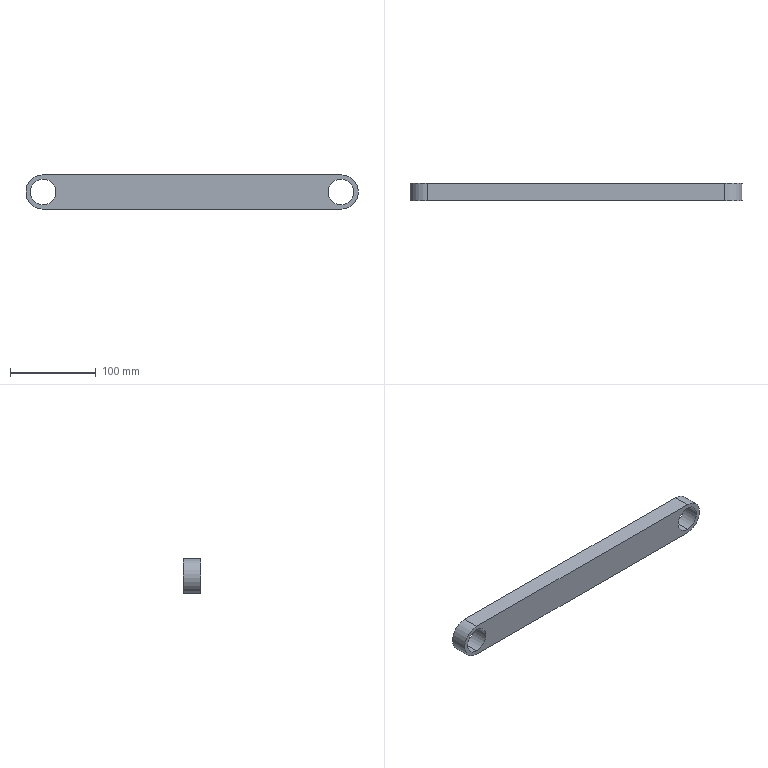Part | STEP file | LM-05-1256_default | 1 solid | 10 faces | box 387.07 x 20 x 40 mm | volume 274514 mm3 | cylinder 6 | plane 4 | commonest cylinder face diameters 30 x4 40 x2
STEP:
#1=CARTESIAN_POINT('',(0.,0.,0.));
#2=DIRECTION('',(0.,0.,1.));
#3=DIRECTION('',(1.,0.,0.));
#4=AXIS2_PLACEMENT_3D('',#1,#2,#3);
#5=CARTESIAN_POINT('',(-173.535,10.,-15.));
#6=VERTEX_POINT('',#5);
#7=CARTESIAN_POINT('',(-173.535,-10.,-15.));
#8=VERTEX_POINT('',#7);
#9=CARTESIAN_POINT('',(-173.535,10.,-15.));
#10=DIRECTION('',(0.,-1.,0.));
#11=VECTOR('',#10,1.);
#12=LINE('',#9,#11);
#13=CARTESIAN_POINT('',(-173.535,10.,0.));
#14=DIRECTION('',(0.,-1.,0.));
#15=DIRECTION('',(0.,0.,-1.));
#16=AXIS2_PLACEMENT_3D('',#13,#14,#15);
#17=CYLINDRICAL_SURFACE('',#16,15.);
#18=CARTESIAN_POINT('',(6.283,0.));
#19=DIRECTION('',(0.,1.));
#20=VECTOR('',#19,1.);
#21=LINE('',#18,#20);
#22=(GEOMETRIC_REPRESENTATION_CONTEXT(2)PARAMETRIC_REPRESENTATION_CONTEXT()REPRESENTATION_CONTEXT('',''));
#23=DEFINITIONAL_REPRESENTATION('',(#21),#22);
#24=PCURVE('',#17,#23);
#25=CARTESIAN_POINT('',(-173.535,10.,0.));
#26=DIRECTION('',(0.,-1.,0.));
#27=DIRECTION('',(0.,0.,-1.));
#28=AXIS2_PLACEMENT_3D('',#25,#26,#27);
#29=CYLINDRICAL_SURFACE('',#28,15.);
#30=CARTESIAN_POINT('',(0.,0.));
#31=DIRECTION('',(0.,1.));
#32=VECTOR('',#31,1.);
#33=LINE('',#30,#32);
#34=(GEOMETRIC_REPRESENTATION_CONTEXT(2)PARAMETRIC_REPRESENTATION_CONTEXT()REPRESENTATION_CONTEXT('',''));
#35=DEFINITIONAL_REPRESENTATION('',(#33),#34);
#36=PCURVE('',#29,#35);
#37=SURFACE_CURVE('',#12,(#24,#36),.PCURVE_S1.);
#38=EDGE_CURVE('',#6,#8,#37,.T.);
#39=ORIENTED_EDGE('',*,*,#38,.T.);
#40=CARTESIAN_POINT('',(-173.535,-10.,15.));
#41=VERTEX_POINT('',#40);
#42=CARTESIAN_POINT('',(-173.535,-10.,0.));
#43=DIRECTION('',(0.,-1.,0.));
#44=DIRECTION('',(0.,0.,1.));
#45=AXIS2_PLACEMENT_3D('',#42,#43,#44);
#46=CIRCLE('',#45,15.);
#47=CARTESIAN_POINT('',(3.142,20.));
#48=DIRECTION('',(1.,0.));
#49=VECTOR('',#48,1.);
#50=LINE('',#47,#49);
#51=(GEOMETRIC_REPRESENTATION_CONTEXT(2)PARAMETRIC_REPRESENTATION_CONTEXT()REPRESENTATION_CONTEXT('',''));
#52=DEFINITIONAL_REPRESENTATION('',(#50),#51);
#53=PCURVE('',#17,#52);
#54=CARTESIAN_POINT('',(-173.535,-10.,0.));
#55=DIRECTION('',(0.,-1.,0.));
#56=DIRECTION('',(0.,0.,-1.));
#57=AXIS2_PLACEMENT_3D('',#54,#55,#56);
#58=PLANE('',#57);
#59=CARTESIAN_POINT('',(0.,0.));
#60=DIRECTION('',(-1.,0.));
#61=AXIS2_PLACEMENT_2D('',#59,#60);
#62=CIRCLE('',#61,15.);
#63=(GEOMETRIC_REPRESENTATION_CONTEXT(2)PARAMETRIC_REPRESENTATION_CONTEXT()REPRESENTATION_CONTEXT('',''));
#64=DEFINITIONAL_REPRESENTATION('',(#62),#63);
#65=PCURVE('',#58,#64);
#66=SURFACE_CURVE('',#46,(#53,#65),.PCURVE_S1.);
#67=EDGE_CURVE('',#41,#8,#66,.T.);
#68=ORIENTED_EDGE('',*,*,#67,.F.);
#69=CARTESIAN_POINT('',(-173.535,10.,15.));
#70=VERTEX_POINT('',#69);
#71=CARTESIAN_POINT('',(-173.535,10.,15.));
#72=DIRECTION('',(0.,-1.,0.));
#73=VECTOR('',#72,1.);
#74=LINE('',#71,#73);
#75=CARTESIAN_POINT('',(3.142,0.));
#76=DIRECTION('',(0.,1.));
#77=VECTOR('',#76,1.);
#78=LINE('',#75,#77);
#79=(GEOMETRIC_REPRESENTATION_CONTEXT(2)PARAMETRIC_REPRESENTATION_CONTEXT()REPRESENTATION_CONTEXT('',''));
#80=DEFINITIONAL_REPRESENTATION('',(#78),#79);
#81=PCURVE('',#17,#80);
#82=CARTESIAN_POINT('',(3.142,0.));
#83=DIRECTION('',(0.,1.));
#84=VECTOR('',#83,1.);
#85=LINE('',#82,#84);
#86=(GEOMETRIC_REPRESENTATION_CONTEXT(2)PARAMETRIC_REPRESENTATION_CONTEXT()REPRESENTATION_CONTEXT('',''));
#87=DEFINITIONAL_REPRESENTATION('',(#85),#86);
#88=PCURVE('',#29,#87);
#89=SURFACE_CURVE('',#74,(#81,#88),.PCURVE_S1.);
#90=EDGE_CURVE('',#70,#41,#89,.T.);
#91=ORIENTED_EDGE('',*,*,#90,.F.);
#92=CARTESIAN_POINT('',(-173.535,10.,0.));
#93=DIRECTION('',(0.,-1.,0.));
#94=DIRECTION('',(0.,0.,1.));
#95=AXIS2_PLACEMENT_3D('',#92,#93,#94);
#96=CIRCLE('',#95,15.);
#97=CARTESIAN_POINT('',(3.142,0.));
#98=DIRECTION('',(1.,0.));
#99=VECTOR('',#98,1.);
#100=LINE('',#97,#99);
#101=(GEOMETRIC_REPRESENTATION_CONTEXT(2)PARAMETRIC_REPRESENTATION_CONTEXT()REPRESENTATION_CONTEXT('',''));
#102=DEFINITIONAL_REPRESENTATION('',(#100),#101);
#103=PCURVE('',#17,#102);
#104=CARTESIAN_POINT('',(-173.535,10.,0.));
#105=DIRECTION('',(0.,-1.,0.));
#106=DIRECTION('',(0.,0.,-1.));
#107=AXIS2_PLACEMENT_3D('',#104,#105,#106);
#108=PLANE('',#107);
#109=CARTESIAN_POINT('',(0.,0.));
#110=DIRECTION('',(-1.,0.));
#111=AXIS2_PLACEMENT_2D('',#109,#110);
#112=CIRCLE('',#111,15.);
#113=(GEOMETRIC_REPRESENTATION_CONTEXT(2)PARAMETRIC_REPRESENTATION_CONTEXT()REPRESENTATION_CONTEXT('',''));
#114=DEFINITIONAL_REPRESENTATION('',(#112),#113);
#115=PCURVE('',#108,#114);
#116=SURFACE_CURVE('',#96,(#103,#115),.PCURVE_S1.);
#117=EDGE_CURVE('',#70,#6,#116,.T.);
#118=ORIENTED_EDGE('',*,*,#117,.T.);
#119=EDGE_LOOP('',(#39,#68,#91,#118));
#120=FACE_BOUND('',#119,.F.);
#121=ADVANCED_FACE('',(#120),#17,.F.);
#122=CARTESIAN_POINT('',(173.535,10.,-15.));
#123=VERTEX_POINT('',#122);
#124=CARTESIAN_POINT('',(173.535,-10.,-15.));
#125=VERTEX_POINT('',#124);
#126=CARTESIAN_POINT('',(173.535,10.,-15.));
#127=DIRECTION('',(0.,-1.,0.));
#128=VECTOR('',#127,1.);
#129=LINE('',#126,#128);
#130=CARTESIAN_POINT('',(173.535,10.,0.));
#131=DIRECTION('',(0.,-1.,0.));
#132=DIRECTION('',(0.,0.,-1.));
#133=AXIS2_PLACEMENT_3D('',#130,#131,#132);
#134=CYLINDRICAL_SURFACE('',#133,15.);
#135=CARTESIAN_POINT('',(6.283,0.));
#136=DIRECTION('',(0.,1.));
#137=VECTOR('',#136,1.);
#138=LINE('',#135,#137);
#139=(GEOMETRIC_REPRESENTATION_CONTEXT(2)PARAMETRIC_REPRESENTATION_CONTEXT()REPRESENTATION_CONTEXT('',''));
#140=DEFINITIONAL_REPRESENTATION('',(#138),#139);
#141=PCURVE('',#134,#140);
#142=CARTESIAN_POINT('',(173.535,10.,0.));
#143=DIRECTION('',(0.,-1.,0.));
#144=DIRECTION('',(0.,0.,-1.));
#145=AXIS2_PLACEMENT_3D('',#142,#143,#144);
#146=CYLINDRICAL_SURFACE('',#145,15.);
#147=CARTESIAN_POINT('',(0.,0.));
#148=DIRECTION('',(0.,1.));
#149=VECTOR('',#148,1.);
#150=LINE('',#147,#149);
#151=(GEOMETRIC_REPRESENTATION_CONTEXT(2)PARAMETRIC_REPRESENTATION_CONTEXT()REPRESENTATION_CONTEXT('',''));
#152=DEFINITIONAL_REPRESENTATION('',(#150),#151);
#153=PCURVE('',#146,#152);
#154=SURFACE_CURVE('',#129,(#141,#153),.PCURVE_S1.);
#155=EDGE_CURVE('',#123,#125,#154,.T.);
#156=ORIENTED_EDGE('',*,*,#155,.T.);
#157=CARTESIAN_POINT('',(173.535,-10.,15.));
#158=VERTEX_POINT('',#157);
#159=CARTESIAN_POINT('',(173.535,-10.,0.));
#160=DIRECTION('',(0.,-1.,0.));
#161=DIRECTION('',(0.,0.,1.));
#162=AXIS2_PLACEMENT_3D('',#159,#160,#161);
#163=CIRCLE('',#162,15.);
#164=CARTESIAN_POINT('',(3.142,20.));
#165=DIRECTION('',(1.,0.));
#166=VECTOR('',#165,1.);
#167=LINE('',#164,#166);
#168=(GEOMETRIC_REPRESENTATION_CONTEXT(2)PARAMETRIC_REPRESENTATION_CONTEXT()REPRESENTATION_CONTEXT('',''));
#169=DEFINITIONAL_REPRESENTATION('',(#167),#168);
#170=PCURVE('',#134,#169);
#171=CARTESIAN_POINT('',(0.,347.07));
#172=DIRECTION('',(-1.,0.));
#173=AXIS2_PLACEMENT_2D('',#171,#172);
#174=CIRCLE('',#173,15.);
#175=(GEOMETRIC_REPRESENTATION_CONTEXT(2)PARAMETRIC_REPRESENTATION_CONTEXT()REPRESENTATION_CONTEXT('',''));
#176=DEFINITIONAL_REPRESENTATION('',(#174),#175);
#177=PCURVE('',#58,#176);
#178=SURFACE_CURVE('',#163,(#170,#177),.PCURVE_S1.);
#179=EDGE_CURVE('',#158,#125,#178,.T.);
#180=ORIENTED_EDGE('',*,*,#179,.F.);
#181=CARTESIAN_POINT('',(173.535,10.,15.));
#182=VERTEX_POINT('',#181);
#183=CARTESIAN_POINT('',(173.535,10.,15.));
#184=DIRECTION('',(0.,-1.,0.));
#185=VECTOR('',#184,1.);
#186=LINE('',#183,#185);
#187=CARTESIAN_POINT('',(3.142,0.));
#188=DIRECTION('',(0.,1.));
#189=VECTOR('',#188,1.);
#190=LINE('',#187,#189);
#191=(GEOMETRIC_REPRESENTATION_CONTEXT(2)PARAMETRIC_REPRESENTATION_CONTEXT()REPRESENTATION_CONTEXT('',''));
#192=DEFINITIONAL_REPRESENTATION('',(#190),#191);
#193=PCURVE('',#134,#192);
#194=CARTESIAN_POINT('',(3.142,0.));
#195=DIRECTION('',(0.,1.));
#196=VECTOR('',#195,1.);
#197=LINE('',#194,#196);
#198=(GEOMETRIC_REPRESENTATION_CONTEXT(2)PARAMETRIC_REPRESENTATION_CONTEXT()REPRESENTATION_CONTEXT('',''));
#199=DEFINITIONAL_REPRESENTATION('',(#197),#198);
#200=PCURVE('',#146,#199);
#201=SURFACE_CURVE('',#186,(#193,#200),.PCURVE_S1.);
#202=EDGE_CURVE('',#182,#158,#201,.T.);
#203=ORIENTED_EDGE('',*,*,#202,.F.);
#204=CARTESIAN_POINT('',(173.535,10.,0.));
#205=DIRECTION('',(0.,-1.,0.));
#206=DIRECTION('',(0.,0.,1.));
#207=AXIS2_PLACEMENT_3D('',#204,#205,#206);
#208=CIRCLE('',#207,15.);
#209=CARTESIAN_POINT('',(3.142,0.));
#210=DIRECTION('',(1.,0.));
#211=VECTOR('',#210,1.);
#212=LINE('',#209,#211);
#213=(GEOMETRIC_REPRESENTATION_CONTEXT(2)PARAMETRIC_REPRESENTATION_CONTEXT()REPRESENTATION_CONTEXT('',''));
#214=DEFINITIONAL_REPRESENTATION('',(#212),#213);
#215=PCURVE('',#134,#214);
#216=CARTESIAN_POINT('',(0.,347.07));
#217=DIRECTION('',(-1.,0.));
#218=AXIS2_PLACEMENT_2D('',#216,#217);
#219=CIRCLE('',#218,15.);
#220=(GEOMETRIC_REPRESENTATION_CONTEXT(2)PARAMETRIC_REPRESENTATION_CONTEXT()REPRESENTATION_CONTEXT('',''));
#221=DEFINITIONAL_REPRESENTATION('',(#219),#220);
#222=PCURVE('',#108,#221);
#223=SURFACE_CURVE('',#208,(#215,#222),.PCURVE_S1.);
#224=EDGE_CURVE('',#182,#123,#223,.T.);
#225=ORIENTED_EDGE('',*,*,#224,.T.);
#226=EDGE_LOOP('',(#156,#180,#203,#225));
#227=FACE_BOUND('',#226,.F.);
#228=ADVANCED_FACE('',(#227),#134,.F.);
#229=CARTESIAN_POINT('',(-173.535,-10.,20.));
#230=VERTEX_POINT('',#229);
#231=CARTESIAN_POINT('',(-173.535,-10.,-20.));
#232=VERTEX_POINT('',#231);
#233=CARTESIAN_POINT('',(-173.535,-10.,0.));
#234=DIRECTION('',(0.,-1.,0.));
#235=DIRECTION('',(0.,0.,-1.));
#236=AXIS2_PLACEMENT_3D('',#233,#234,#235);
#237=CIRCLE('',#236,20.);
#238=CARTESIAN_POINT('',(-173.535,10.,0.));
#239=DIRECTION('',(0.,-1.,0.));
#240=DIRECTION('',(0.,0.,-1.));
#241=AXIS2_PLACEMENT_3D('',#238,#239,#240);
#242=CYLINDRICAL_SURFACE('',#241,20.);
#243=CARTESIAN_POINT('',(0.,20.));
#244=DIRECTION('',(1.,0.));
#245=VECTOR('',#244,1.);
#246=LINE('',#243,#245);
#247=(GEOMETRIC_REPRESENTATION_CONTEXT(2)PARAMETRIC_REPRESENTATION_CONTEXT()REPRESENTATION_CONTEXT('',''));
#248=DEFINITIONAL_REPRESENTATION('',(#246),#247);
#249=PCURVE('',#242,#248);
#250=CARTESIAN_POINT('',(0.,0.));
#251=DIRECTION('',(1.,0.));
#252=AXIS2_PLACEMENT_2D('',#250,#251);
#253=CIRCLE('',#252,20.);
#254=(GEOMETRIC_REPRESENTATION_CONTEXT(2)PARAMETRIC_REPRESENTATION_CONTEXT()REPRESENTATION_CONTEXT('',''));
#255=DEFINITIONAL_REPRESENTATION('',(#253),#254);
#256=PCURVE('',#58,#255);
#257=SURFACE_CURVE('',#237,(#249,#256),.PCURVE_S1.);
#258=EDGE_CURVE('',#230,#232,#257,.T.);
#259=ORIENTED_EDGE('',*,*,#258,.F.);
#260=CARTESIAN_POINT('',(-173.535,10.,20.));
#261=VERTEX_POINT('',#260);
#262=CARTESIAN_POINT('',(-173.535,10.,20.));
#263=DIRECTION('',(0.,-1.,0.));
#264=VECTOR('',#263,1.);
#265=LINE('',#262,#264);
#266=CARTESIAN_POINT('',(3.142,0.));
#267=DIRECTION('',(0.,1.));
#268=VECTOR('',#267,1.);
#269=LINE('',#266,#268);
#270=(GEOMETRIC_REPRESENTATION_CONTEXT(2)PARAMETRIC_REPRESENTATION_CONTEXT()REPRESENTATION_CONTEXT('',''));
#271=DEFINITIONAL_REPRESENTATION('',(#269),#270);
#272=PCURVE('',#242,#271);
#273=CARTESIAN_POINT('',(173.535,10.,20.));
#274=DIRECTION('',(0.,0.,1.));
#275=DIRECTION('',(1.,0.,0.));
#276=AXIS2_PLACEMENT_3D('',#273,#274,#275);
#277=PLANE('',#276);
#278=CARTESIAN_POINT('',(-347.07,0.));
#279=DIRECTION('',(0.,-1.));
#280=VECTOR('',#279,1.);
#281=LINE('',#278,#280);
#282=(GEOMETRIC_REPRESENTATION_CONTEXT(2)PARAMETRIC_REPRESENTATION_CONTEXT()REPRESENTATION_CONTEXT('',''));
#283=DEFINITIONAL_REPRESENTATION('',(#281),#282);
#284=PCURVE('',#277,#283);
#285=SURFACE_CURVE('',#265,(#272,#284),.PCURVE_S1.);
#286=EDGE_CURVE('',#261,#230,#285,.T.);
#287=ORIENTED_EDGE('',*,*,#286,.F.);
#288=CARTESIAN_POINT('',(-173.535,10.,-20.));
#289=VERTEX_POINT('',#288);
#290=CARTESIAN_POINT('',(-173.535,10.,0.));
#291=DIRECTION('',(0.,-1.,0.));
#292=DIRECTION('',(0.,0.,-1.));
#293=AXIS2_PLACEMENT_3D('',#290,#291,#292);
#294=CIRCLE('',#293,20.);
#295=CARTESIAN_POINT('',(0.,0.));
#296=DIRECTION('',(1.,0.));
#297=VECTOR('',#296,1.);
#298=LINE('',#295,#297);
#299=(GEOMETRIC_REPRESENTATION_CONTEXT(2)PARAMETRIC_REPRESENTATION_CONTEXT()REPRESENTATION_CONTEXT('',''));
#300=DEFINITIONAL_REPRESENTATION('',(#298),#299);
#301=PCURVE('',#242,#300);
#302=CARTESIAN_POINT('',(0.,0.));
#303=DIRECTION('',(1.,0.));
#304=AXIS2_PLACEMENT_2D('',#302,#303);
#305=CIRCLE('',#304,20.);
#306=(GEOMETRIC_REPRESENTATION_CONTEXT(2)PARAMETRIC_REPRESENTATION_CONTEXT()REPRESENTATION_CONTEXT('',''));
#307=DEFINITIONAL_REPRESENTATION('',(#305),#306);
#308=PCURVE('',#108,#307);
#309=SURFACE_CURVE('',#294,(#301,#308),.PCURVE_S1.);
#310=EDGE_CURVE('',#261,#289,#309,.T.);
#311=ORIENTED_EDGE('',*,*,#310,.T.);
#312=CARTESIAN_POINT('',(-173.535,10.,-20.));
#313=DIRECTION('',(0.,-1.,0.));
#314=VECTOR('',#313,1.);
#315=LINE('',#312,#314);
#316=CARTESIAN_POINT('',(6.283,0.));
#317=DIRECTION('',(0.,1.));
#318=VECTOR('',#317,1.);
#319=LINE('',#316,#318);
#320=(GEOMETRIC_REPRESENTATION_CONTEXT(2)PARAMETRIC_REPRESENTATION_CONTEXT()REPRESENTATION_CONTEXT('',''));
#321=DEFINITIONAL_REPRESENTATION('',(#319),#320);
#322=PCURVE('',#242,#321);
#323=CARTESIAN_POINT('',(-173.535,10.,-20.));
#324=DIRECTION('',(0.,0.,-1.));
#325=DIRECTION('',(-1.,0.,0.));
#326=AXIS2_PLACEMENT_3D('',#323,#324,#325);
#327=PLANE('',#326);
#328=CARTESIAN_POINT('',(0.,0.));
#329=DIRECTION('',(0.,-1.));
#330=VECTOR('',#329,1.);
#331=LINE('',#328,#330);
#332=(GEOMETRIC_REPRESENTATION_CONTEXT(2)PARAMETRIC_REPRESENTATION_CONTEXT()REPRESENTATION_CONTEXT('',''));
#333=DEFINITIONAL_REPRESENTATION('',(#331),#332);
#334=PCURVE('',#327,#333);
#335=SURFACE_CURVE('',#315,(#322,#334),.PCURVE_S1.);
#336=EDGE_CURVE('',#289,#232,#335,.T.);
#337=ORIENTED_EDGE('',*,*,#336,.T.);
#338=EDGE_LOOP('',(#259,#287,#311,#337));
#339=FACE_BOUND('',#338,.T.);
#340=ADVANCED_FACE('',(#339),#242,.T.);
#341=CARTESIAN_POINT('',(173.535,-10.,20.));
#342=VERTEX_POINT('',#341);
#343=CARTESIAN_POINT('',(173.535,-10.,20.));
#344=DIRECTION('',(-1.,0.,0.));
#345=VECTOR('',#344,1.);
#346=LINE('',#343,#345);
#347=CARTESIAN_POINT('',(0.,-20.));
#348=DIRECTION('',(-1.,0.));
#349=VECTOR('',#348,1.);
#350=LINE('',#347,#349);
#351=(GEOMETRIC_REPRESENTATION_CONTEXT(2)PARAMETRIC_REPRESENTATION_CONTEXT()REPRESENTATION_CONTEXT('',''));
#352=DEFINITIONAL_REPRESENTATION('',(#350),#351);
#353=PCURVE('',#277,#352);
#354=CARTESIAN_POINT('',(-20.,347.07));
#355=DIRECTION('',(0.,-1.));
#356=VECTOR('',#355,1.);
#357=LINE('',#354,#356);
#358=(GEOMETRIC_REPRESENTATION_CONTEXT(2)PARAMETRIC_REPRESENTATION_CONTEXT()REPRESENTATION_CONTEXT('',''));
#359=DEFINITIONAL_REPRESENTATION('',(#357),#358);
#360=PCURVE('',#58,#359);
#361=SURFACE_CURVE('',#346,(#353,#360),.PCURVE_S1.);
#362=EDGE_CURVE('',#342,#230,#361,.T.);
#363=ORIENTED_EDGE('',*,*,#362,.F.);
#364=CARTESIAN_POINT('',(173.535,10.,20.));
#365=VERTEX_POINT('',#364);
#366=CARTESIAN_POINT('',(173.535,10.,20.));
#367=DIRECTION('',(0.,-1.,0.));
#368=VECTOR('',#367,1.);
#369=LINE('',#366,#368);
#370=CARTESIAN_POINT('',(0.,0.));
#371=DIRECTION('',(0.,-1.));
#372=VECTOR('',#371,1.);
#373=LINE('',#370,#372);
#374=(GEOMETRIC_REPRESENTATION_CONTEXT(2)PARAMETRIC_REPRESENTATION_CONTEXT()REPRESENTATION_CONTEXT('',''));
#375=DEFINITIONAL_REPRESENTATION('',(#373),#374);
#376=PCURVE('',#277,#375);
#377=CARTESIAN_POINT('',(173.535,10.,0.));
#378=DIRECTION('',(0.,-1.,0.));
#379=DIRECTION('',(0.,0.,-1.));
#380=AXIS2_PLACEMENT_3D('',#377,#378,#379);
#381=CYLINDRICAL_SURFACE('',#380,20.);
#382=CARTESIAN_POINT('',(3.142,0.));
#383=DIRECTION('',(0.,1.));
#384=VECTOR('',#383,1.);
#385=LINE('',#382,#384);
#386=(GEOMETRIC_REPRESENTATION_CONTEXT(2)PARAMETRIC_REPRESENTATION_CONTEXT()REPRESENTATION_CONTEXT('',''));
#387=DEFINITIONAL_REPRESENTATION('',(#385),#386);
#388=PCURVE('',#381,#387);
#389=SURFACE_CURVE('',#369,(#376,#388),.PCURVE_S1.);
#390=EDGE_CURVE('',#365,#342,#389,.T.);
#391=ORIENTED_EDGE('',*,*,#390,.F.);
#392=CARTESIAN_POINT('',(173.535,10.,20.));
#393=DIRECTION('',(-1.,0.,0.));
#394=VECTOR('',#393,1.);
#395=LINE('',#392,#394);
#396=CARTESIAN_POINT('',(0.,0.));
#397=DIRECTION('',(-1.,0.));
#398=VECTOR('',#397,1.);
#399=LINE('',#396,#398);
#400=(GEOMETRIC_REPRESENTATION_CONTEXT(2)PARAMETRIC_REPRESENTATION_CONTEXT()REPRESENTATION_CONTEXT('',''));
#401=DEFINITIONAL_REPRESENTATION('',(#399),#400);
#402=PCURVE('',#277,#401);
#403=CARTESIAN_POINT('',(-20.,347.07));
#404=DIRECTION('',(0.,-1.));
#405=VECTOR('',#404,1.);
#406=LINE('',#403,#405);
#407=(GEOMETRIC_REPRESENTATION_CONTEXT(2)PARAMETRIC_REPRESENTATION_CONTEXT()REPRESENTATION_CONTEXT('',''));
#408=DEFINITIONAL_REPRESENTATION('',(#406),#407);
#409=PCURVE('',#108,#408);
#410=SURFACE_CURVE('',#395,(#402,#409),.PCURVE_S1.);
#411=EDGE_CURVE('',#365,#261,#410,.T.);
#412=ORIENTED_EDGE('',*,*,#411,.T.);
#413=ORIENTED_EDGE('',*,*,#286,.T.);
#414=EDGE_LOOP('',(#363,#391,#412,#413));
#415=FACE_BOUND('',#414,.T.);
#416=ADVANCED_FACE('',(#415),#277,.T.);
#417=CARTESIAN_POINT('',(173.535,-10.,-20.));
#418=VERTEX_POINT('',#417);
#419=CARTESIAN_POINT('',(173.535,-10.,0.));
#420=DIRECTION('',(0.,-1.,0.));
#421=DIRECTION('',(0.,0.,-1.));
#422=AXIS2_PLACEMENT_3D('',#419,#420,#421);
#423=CIRCLE('',#422,20.);
#424=CARTESIAN_POINT('',(0.,20.));
#425=DIRECTION('',(1.,0.));
#426=VECTOR('',#425,1.);
#427=LINE('',#424,#426);
#428=(GEOMETRIC_REPRESENTATION_CONTEXT(2)PARAMETRIC_REPRESENTATION_CONTEXT()REPRESENTATION_CONTEXT('',''));
#429=DEFINITIONAL_REPRESENTATION('',(#427),#428);
#430=PCURVE('',#381,#429);
#431=CARTESIAN_POINT('',(0.,347.07));
#432=DIRECTION('',(1.,0.));
#433=AXIS2_PLACEMENT_2D('',#431,#432);
#434=CIRCLE('',#433,20.);
#435=(GEOMETRIC_REPRESENTATION_CONTEXT(2)PARAMETRIC_REPRESENTATION_CONTEXT()REPRESENTATION_CONTEXT('',''));
#436=DEFINITIONAL_REPRESENTATION('',(#434),#435);
#437=PCURVE('',#58,#436);
#438=SURFACE_CURVE('',#423,(#430,#437),.PCURVE_S1.);
#439=EDGE_CURVE('',#418,#342,#438,.T.);
#440=ORIENTED_EDGE('',*,*,#439,.F.);
#441=CARTESIAN_POINT('',(173.535,10.,-20.));
#442=VERTEX_POINT('',#441);
#443=CARTESIAN_POINT('',(173.535,10.,-20.));
#444=DIRECTION('',(0.,-1.,0.));
#445=VECTOR('',#444,1.);
#446=LINE('',#443,#445);
#447=CARTESIAN_POINT('',(0.,0.));
#448=DIRECTION('',(0.,1.));
#449=VECTOR('',#448,1.);
#450=LINE('',#447,#449);
#451=(GEOMETRIC_REPRESENTATION_CONTEXT(2)PARAMETRIC_REPRESENTATION_CONTEXT()REPRESENTATION_CONTEXT('',''));
#452=DEFINITIONAL_REPRESENTATION('',(#450),#451);
#453=PCURVE('',#381,#452);
#454=CARTESIAN_POINT('',(-347.07,0.));
#455=DIRECTION('',(0.,-1.));
#456=VECTOR('',#455,1.);
#457=LINE('',#454,#456);
#458=(GEOMETRIC_REPRESENTATION_CONTEXT(2)PARAMETRIC_REPRESENTATION_CONTEXT()REPRESENTATION_CONTEXT('',''));
#459=DEFINITIONAL_REPRESENTATION('',(#457),#458);
#460=PCURVE('',#327,#459);
#461=SURFACE_CURVE('',#446,(#453,#460),.PCURVE_S1.);
#462=EDGE_CURVE('',#442,#418,#461,.T.);
#463=ORIENTED_EDGE('',*,*,#462,.F.);
#464=CARTESIAN_POINT('',(173.535,10.,0.));
#465=DIRECTION('',(0.,-1.,0.));
#466=DIRECTION('',(0.,0.,-1.));
#467=AXIS2_PLACEMENT_3D('',#464,#465,#466);
#468=CIRCLE('',#467,20.);
#469=CARTESIAN_POINT('',(0.,0.));
#470=DIRECTION('',(1.,0.));
#471=VECTOR('',#470,1.);
#472=LINE('',#469,#471);
#473=(GEOMETRIC_REPRESENTATION_CONTEXT(2)PARAMETRIC_REPRESENTATION_CONTEXT()REPRESENTATION_CONTEXT('',''));
#474=DEFINITIONAL_REPRESENTATION('',(#472),#473);
#475=PCURVE('',#381,#474);
#476=CARTESIAN_POINT('',(0.,347.07));
#477=DIRECTION('',(1.,0.));
#478=AXIS2_PLACEMENT_2D('',#476,#477);
#479=CIRCLE('',#478,20.);
#480=(GEOMETRIC_REPRESENTATION_CONTEXT(2)PARAMETRIC_REPRESENTATION_CONTEXT()REPRESENTATION_CONTEXT('',''));
#481=DEFINITIONAL_REPRESENTATION('',(#479),#480);
#482=PCURVE('',#108,#481);
#483=SURFACE_CURVE('',#468,(#475,#482),.PCURVE_S1.);
#484=EDGE_CURVE('',#442,#365,#483,.T.);
#485=ORIENTED_EDGE('',*,*,#484,.T.);
#486=ORIENTED_EDGE('',*,*,#390,.T.);
#487=EDGE_LOOP('',(#440,#463,#485,#486));
#488=FACE_BOUND('',#487,.T.);
#489=ADVANCED_FACE('',(#488),#381,.T.);
#490=CARTESIAN_POINT('',(-173.535,-10.,-20.));
#491=DIRECTION('',(1.,0.,0.));
#492=VECTOR('',#491,1.);
#493=LINE('',#490,#492);
#494=CARTESIAN_POINT('',(0.,-20.));
#495=DIRECTION('',(-1.,0.));
#496=VECTOR('',#495,1.);
#497=LINE('',#494,#496);
#498=(GEOMETRIC_REPRESENTATION_CONTEXT(2)PARAMETRIC_REPRESENTATION_CONTEXT()REPRESENTATION_CONTEXT('',''));
#499=DEFINITIONAL_REPRESENTATION('',(#497),#498);
#500=PCURVE('',#327,#499);
#501=CARTESIAN_POINT('',(20.,0.));
#502=DIRECTION('',(0.,1.));
#503=VECTOR('',#502,1.);
#504=LINE('',#501,#503);
#505=(GEOMETRIC_REPRESENTATION_CONTEXT(2)PARAMETRIC_REPRESENTATION_CONTEXT()REPRESENTATION_CONTEXT('',''));
#506=DEFINITIONAL_REPRESENTATION('',(#504),#505);
#507=PCURVE('',#58,#506);
#508=SURFACE_CURVE('',#493,(#500,#507),.PCURVE_S1.);
#509=EDGE_CURVE('',#232,#418,#508,.T.);
#510=ORIENTED_EDGE('',*,*,#509,.F.);
#511=ORIENTED_EDGE('',*,*,#336,.F.);
#512=CARTESIAN_POINT('',(-173.535,10.,-20.));
#513=DIRECTION('',(1.,0.,0.));
#514=VECTOR('',#513,1.);
#515=LINE('',#512,#514);
#516=CARTESIAN_POINT('',(0.,0.));
#517=DIRECTION('',(-1.,0.));
#518=VECTOR('',#517,1.);
#519=LINE('',#516,#518);
#520=(GEOMETRIC_REPRESENTATION_CONTEXT(2)PARAMETRIC_REPRESENTATION_CONTEXT()REPRESENTATION_CONTEXT('',''));
#521=DEFINITIONAL_REPRESENTATION('',(#519),#520);
#522=PCURVE('',#327,#521);
#523=CARTESIAN_POINT('',(20.,0.));
#524=DIRECTION('',(0.,1.));
#525=VECTOR('',#524,1.);
#526=LINE('',#523,#525);
#527=(GEOMETRIC_REPRESENTATION_CONTEXT(2)PARAMETRIC_REPRESENTATION_CONTEXT()REPRESENTATION_CONTEXT('',''));
#528=DEFINITIONAL_REPRESENTATION('',(#526),#527);
#529=PCURVE('',#108,#528);
#530=SURFACE_CURVE('',#515,(#522,#529),.PCURVE_S1.);
#531=EDGE_CURVE('',#289,#442,#530,.T.);
#532=ORIENTED_EDGE('',*,*,#531,.T.);
#533=ORIENTED_EDGE('',*,*,#462,.T.);
#534=EDGE_LOOP('',(#510,#511,#532,#533));
#535=FACE_BOUND('',#534,.T.);
#536=ADVANCED_FACE('',(#535),#327,.T.);
#537=CARTESIAN_POINT('',(-173.535,10.,0.));
#538=DIRECTION('',(0.,-1.,0.));
#539=DIRECTION('',(0.,0.,1.));
#540=AXIS2_PLACEMENT_3D('',#537,#538,#539);
#541=CIRCLE('',#540,15.);
#542=CARTESIAN_POINT('',(0.,0.));
#543=DIRECTION('',(-1.,0.));
#544=AXIS2_PLACEMENT_2D('',#542,#543);
#545=CIRCLE('',#544,15.);
#546=(GEOMETRIC_REPRESENTATION_CONTEXT(2)PARAMETRIC_REPRESENTATION_CONTEXT()REPRESENTATION_CONTEXT('',''));
#547=DEFINITIONAL_REPRESENTATION('',(#545),#546);
#548=PCURVE('',#108,#547);
#549=CARTESIAN_POINT('',(-3.142,0.));
#550=DIRECTION('',(1.,0.));
#551=VECTOR('',#550,1.);
#552=LINE('',#549,#551);
#553=(GEOMETRIC_REPRESENTATION_CONTEXT(2)PARAMETRIC_REPRESENTATION_CONTEXT()REPRESENTATION_CONTEXT('',''));
#554=DEFINITIONAL_REPRESENTATION('',(#552),#553);
#555=PCURVE('',#29,#554);
#556=SURFACE_CURVE('',#541,(#548,#555),.PCURVE_S1.);
#557=EDGE_CURVE('',#6,#70,#556,.T.);
#558=ORIENTED_EDGE('',*,*,#557,.T.);
#559=ORIENTED_EDGE('',*,*,#117,.T.);
#560=EDGE_LOOP('',(#558,#559));
#561=FACE_BOUND('',#560,.T.);
#562=CARTESIAN_POINT('',(173.535,10.,0.));
#563=DIRECTION('',(0.,-1.,0.));
#564=DIRECTION('',(0.,0.,1.));
#565=AXIS2_PLACEMENT_3D('',#562,#563,#564);
#566=CIRCLE('',#565,15.);
#567=CARTESIAN_POINT('',(0.,347.07));
#568=DIRECTION('',(-1.,0.));
#569=AXIS2_PLACEMENT_2D('',#567,#568);
#570=CIRCLE('',#569,15.);
#571=(GEOMETRIC_REPRESENTATION_CONTEXT(2)PARAMETRIC_REPRESENTATION_CONTEXT()REPRESENTATION_CONTEXT('',''));
#572=DEFINITIONAL_REPRESENTATION('',(#570),#571);
#573=PCURVE('',#108,#572);
#574=CARTESIAN_POINT('',(-3.142,0.));
#575=DIRECTION('',(1.,0.));
#576=VECTOR('',#575,1.);
#577=LINE('',#574,#576);
#578=(GEOMETRIC_REPRESENTATION_CONTEXT(2)PARAMETRIC_REPRESENTATION_CONTEXT()REPRESENTATION_CONTEXT('',''));
#579=DEFINITIONAL_REPRESENTATION('',(#577),#578);
#580=PCURVE('',#146,#579);
#581=SURFACE_CURVE('',#566,(#573,#580),.PCURVE_S1.);
#582=EDGE_CURVE('',#123,#182,#581,.T.);
#583=ORIENTED_EDGE('',*,*,#582,.T.);
#584=ORIENTED_EDGE('',*,*,#224,.T.);
#585=EDGE_LOOP('',(#583,#584));
#586=FACE_BOUND('',#585,.T.);
#587=ORIENTED_EDGE('',*,*,#310,.F.);
#588=ORIENTED_EDGE('',*,*,#411,.F.);
#589=ORIENTED_EDGE('',*,*,#484,.F.);
#590=ORIENTED_EDGE('',*,*,#531,.F.);
#591=EDGE_LOOP('',(#587,#588,#589,#590));
#592=FACE_BOUND('',#591,.T.);
#593=ADVANCED_FACE('',(#561,#586,#592),#108,.F.);
#594=CARTESIAN_POINT('',(-173.535,-10.,0.));
#595=DIRECTION('',(0.,-1.,0.));
#596=DIRECTION('',(0.,0.,1.));
#597=AXIS2_PLACEMENT_3D('',#594,#595,#596);
#598=CIRCLE('',#597,15.);
#599=CARTESIAN_POINT('',(0.,0.));
#600=DIRECTION('',(-1.,0.));
#601=AXIS2_PLACEMENT_2D('',#599,#600);
#602=CIRCLE('',#601,15.);
#603=(GEOMETRIC_REPRESENTATION_CONTEXT(2)PARAMETRIC_REPRESENTATION_CONTEXT()REPRESENTATION_CONTEXT('',''));
#604=DEFINITIONAL_REPRESENTATION('',(#602),#603);
#605=PCURVE('',#58,#604);
#606=CARTESIAN_POINT('',(-3.142,20.));
#607=DIRECTION('',(1.,0.));
#608=VECTOR('',#607,1.);
#609=LINE('',#606,#608);
#610=(GEOMETRIC_REPRESENTATION_CONTEXT(2)PARAMETRIC_REPRESENTATION_CONTEXT()REPRESENTATION_CONTEXT('',''));
#611=DEFINITIONAL_REPRESENTATION('',(#609),#610);
#612=PCURVE('',#29,#611);
#613=SURFACE_CURVE('',#598,(#605,#612),.PCURVE_S1.);
#614=EDGE_CURVE('',#8,#41,#613,.T.);
#615=ORIENTED_EDGE('',*,*,#614,.F.);
#616=ORIENTED_EDGE('',*,*,#67,.F.);
#617=EDGE_LOOP('',(#615,#616));
#618=FACE_BOUND('',#617,.T.);
#619=CARTESIAN_POINT('',(173.535,-10.,0.));
#620=DIRECTION('',(0.,-1.,0.));
#621=DIRECTION('',(0.,0.,1.));
#622=AXIS2_PLACEMENT_3D('',#619,#620,#621);
#623=CIRCLE('',#622,15.);
#624=CARTESIAN_POINT('',(0.,347.07));
#625=DIRECTION('',(-1.,0.));
#626=AXIS2_PLACEMENT_2D('',#624,#625);
#627=CIRCLE('',#626,15.);
#628=(GEOMETRIC_REPRESENTATION_CONTEXT(2)PARAMETRIC_REPRESENTATION_CONTEXT()REPRESENTATION_CONTEXT('',''));
#629=DEFINITIONAL_REPRESENTATION('',(#627),#628);
#630=PCURVE('',#58,#629);
#631=CARTESIAN_POINT('',(-3.142,20.));
#632=DIRECTION('',(1.,0.));
#633=VECTOR('',#632,1.);
#634=LINE('',#631,#633);
#635=(GEOMETRIC_REPRESENTATION_CONTEXT(2)PARAMETRIC_REPRESENTATION_CONTEXT()REPRESENTATION_CONTEXT('',''));
#636=DEFINITIONAL_REPRESENTATION('',(#634),#635);
#637=PCURVE('',#146,#636);
#638=SURFACE_CURVE('',#623,(#630,#637),.PCURVE_S1.);
#639=EDGE_CURVE('',#125,#158,#638,.T.);
#640=ORIENTED_EDGE('',*,*,#639,.F.);
#641=ORIENTED_EDGE('',*,*,#179,.F.);
#642=EDGE_LOOP('',(#640,#641));
#643=FACE_BOUND('',#642,.T.);
#644=ORIENTED_EDGE('',*,*,#258,.T.);
#645=ORIENTED_EDGE('',*,*,#509,.T.);
#646=ORIENTED_EDGE('',*,*,#439,.T.);
#647=ORIENTED_EDGE('',*,*,#362,.T.);
#648=EDGE_LOOP('',(#644,#645,#646,#647));
#649=FACE_BOUND('',#648,.T.);
#650=ADVANCED_FACE('',(#618,#643,#649),#58,.T.);
#651=ORIENTED_EDGE('',*,*,#639,.F.);
#652=ORIENTED_EDGE('',*,*,#155,.F.);
#653=ORIENTED_EDGE('',*,*,#582,.T.);
#654=ORIENTED_EDGE('',*,*,#202,.T.);
#655=EDGE_LOOP('',(#651,#652,#653,#654));
#656=FACE_BOUND('',#655,.F.);
#657=ADVANCED_FACE('',(#656),#146,.F.);
#658=ORIENTED_EDGE('',*,*,#614,.F.);
#659=ORIENTED_EDGE('',*,*,#38,.F.);
#660=ORIENTED_EDGE('',*,*,#557,.T.);
#661=ORIENTED_EDGE('',*,*,#90,.T.);
#662=EDGE_LOOP('',(#658,#659,#660,#661));
#663=FACE_BOUND('',#662,.F.);
#664=ADVANCED_FACE('',(#663),#29,.F.);
#665=CLOSED_SHELL('',(#121,#228,#340,#416,#489,#536,#593,#650,#657,#664));
#666=MANIFOLD_SOLID_BREP('',#665);
#667=(LENGTH_UNIT()NAMED_UNIT(*)SI_UNIT(.MILLI.,.METRE.));
#668=UNCERTAINTY_MEASURE_WITH_UNIT(LENGTH_MEASURE(0.0000001),#667,'','');
#669=(NAMED_UNIT(*)PLANE_ANGLE_UNIT()SI_UNIT($,.RADIAN.));
#670=(NAMED_UNIT(*)SI_UNIT($,.STERADIAN.)SOLID_ANGLE_UNIT());
#671=(GEOMETRIC_REPRESENTATION_CONTEXT(3)GLOBAL_UNCERTAINTY_ASSIGNED_CONTEXT((#668))GLOBAL_UNIT_ASSIGNED_CONTEXT((#667,#669,#670))REPRESENTATION_CONTEXT('',''));
#672=ADVANCED_BREP_SHAPE_REPRESENTATION('',(#4,#666),#671);